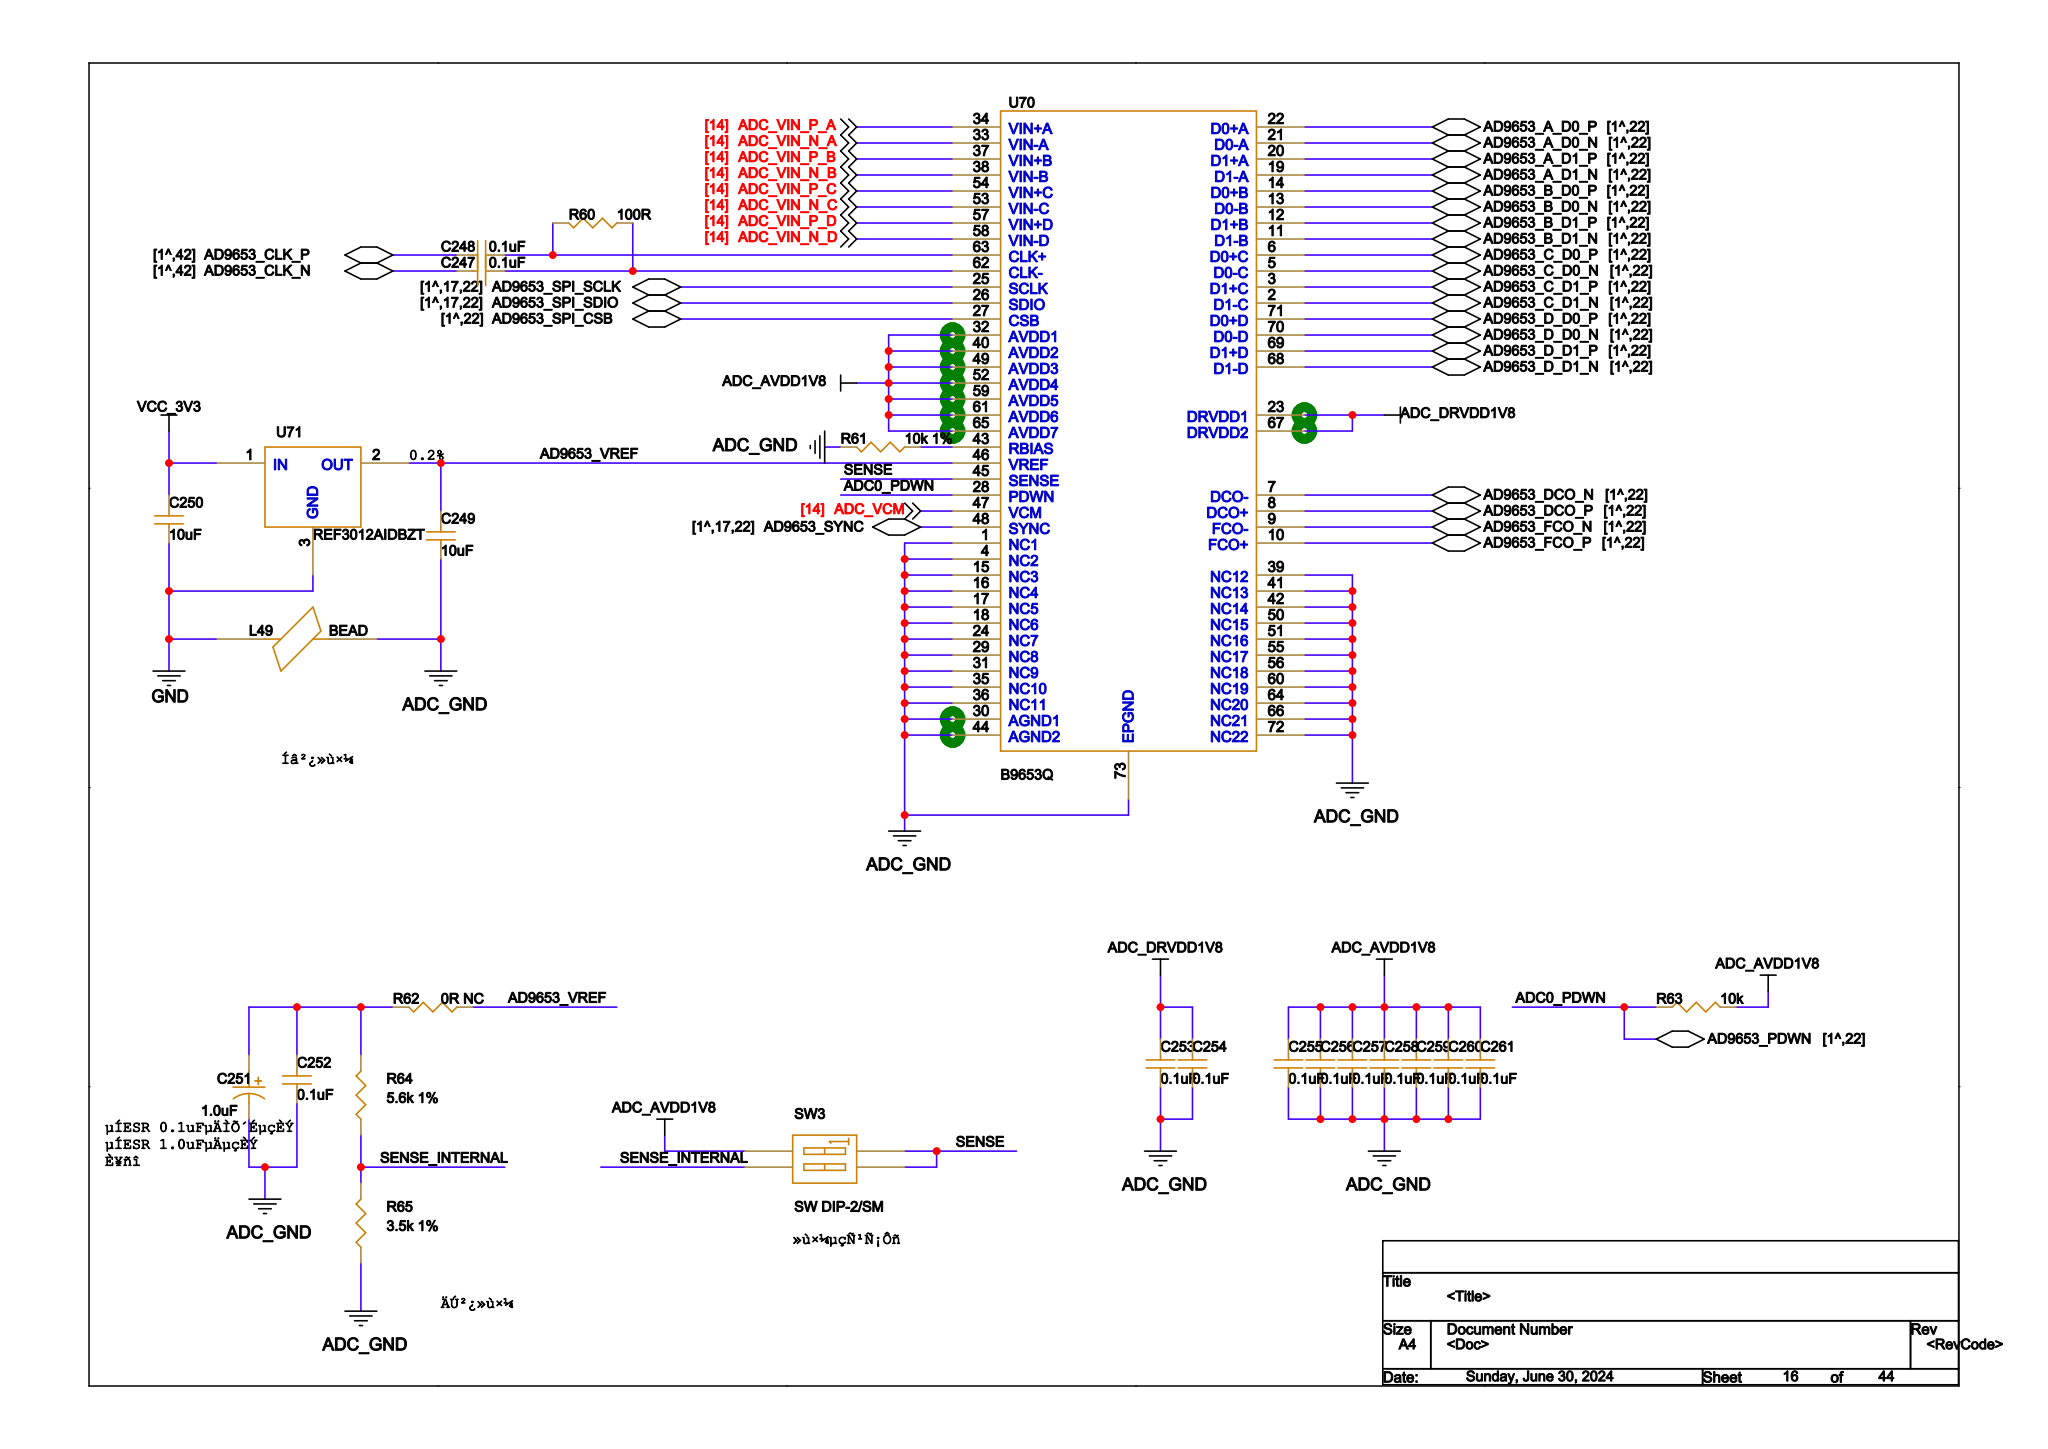Circuit board | Cadence Allegro | 1034 parts | 912 nets | one sheet of the schematic
Parts on this sheet (reference | value | footprint):
C247 | 0.1uF | C0402
C248 | 0.1uF | C0402
C249 | 10uF | C0402
C250 | 10uF | C0402
C251 | 1.0uF | C0402
C252 | 0.1uF | C0402
C253 | 0.1uF | C0402
C254 | 0.1uF | C0402
C255 | 0.1uF | C0402
C256 | 0.1uF | C0402
C257 | 0.1uF | C0402
C258 | 0.1uF | C0402
C259 | 0.1uF | C0402
C260 | 0.1uF | C0402
C261 | 0.1uF | C0402
L49 | BEAD | PZ2012
R60 | 100R | R0402
R61 | 10k 1% | R0402
R62 | 0R NC | R0402
R63 | 10k | R0402
R64 | 5.6k 1% | R0402
R65 | 3.5k 1% | R0402
SW3 | SW DIP-2/SM | SW_2_SOP
U70 | B9653Q | B9653Q_CQFP72
U71 | REF3012AIDBZT | REF3012_SOT23
Nets of these parts (net: part-pin ...):
GND: C250-1 L49-1 U71-3
VCC_3V3: C250-2 U71-1
N186578: C248-2
N186576: C247-2
ADC_GND: C249-1 C251-2 C252-1 C253-1 C254-1 C255-1 C256-1 C257-1 C258-1 C259-1 C260-1 C261-1 L49-2 R61-2 R65-1 U70-1 U70-4 U70-15 U70-16 U70-17 U70-18 U70-24 U70-29 U70-30 U70-31 U70-35 U70-36 U70-39 U70-41 U70-42 U70-44 U70-50 U70-51 U70-55 U70-56 U70-60 U70-64 U70-66 U70-72 U70-73
ADC_AVDD1V8: C255-2 C256-2 C257-2 C258-2 C259-2 C260-2 C261-2 R63-2 SW3-1 U70-32 U70-40 U70-49 U70-52 U70-59 U70-61 U70-65
N111291_D3: C248-1 R60-2 U70-63
N111295_D3: C247-1 R60-1 U70-62
ADC_DRVDD1V8: C253-2 C254-2 U70-67
N187464: R63-1 U70-28
N110707_D3: R61-1 U70-43
SENSE_D3: SW3-3 SW3-4 U70-45
AD9653_VREF_D3: C249-2 R62-1 U71-2 U70-46
N14127011_D3: C251-1 C252-2 R62-2 R64-2
SENSE_INTERNAL_D3: R64-1 R65-2 SW3-2